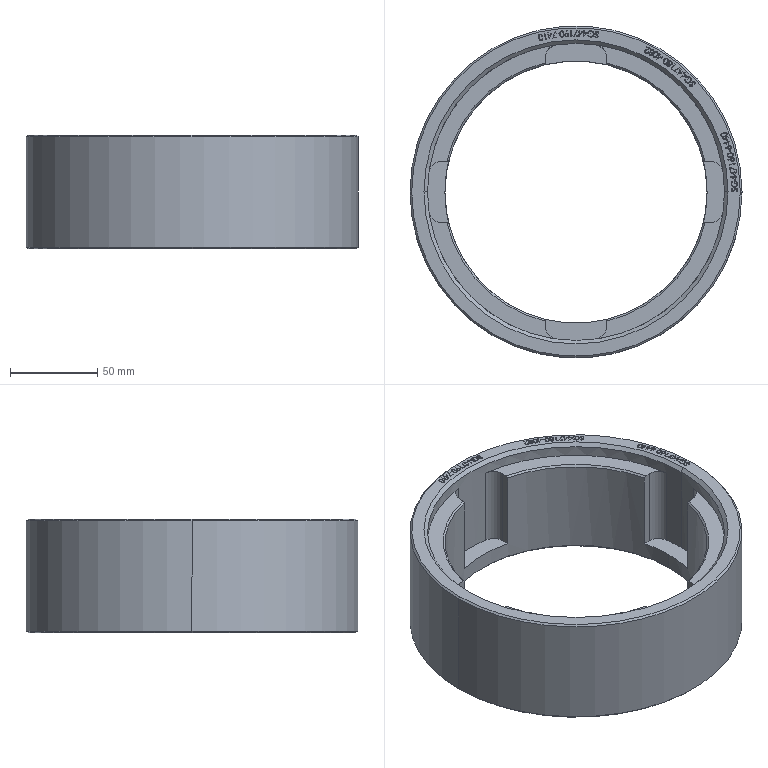Part | STEP file | Gap jig seat-10P30 | 1 solid | 534 faces | box 190 x 190 x 65 mm | volume 588080 mm3 | plane 307 | spline 193 | cylinder 22 | cone 12 | commonest cylinder face diameters 5 x8 15 x8 150 x2 170 x2 190 x2